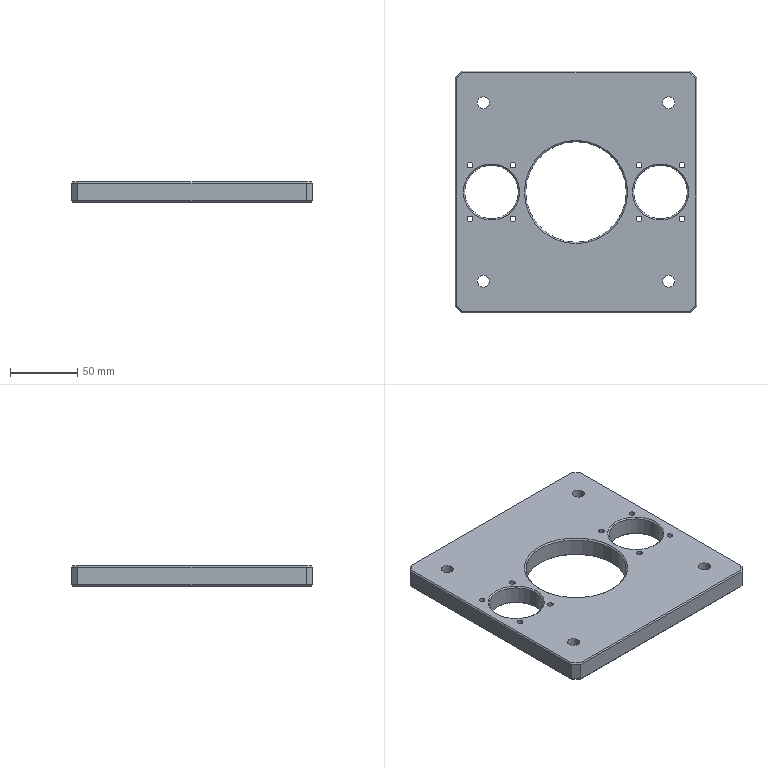Part | STEP file | Bush plate | 1 solid | 80 faces | box 180 x 180 x 15 mm | volume 370713 mm3 | cylinder 38 | plane 30 | cone 12 | commonest cylinder face diameters 4.2 x16 9 x8 15 x8 40 x4 75 x2